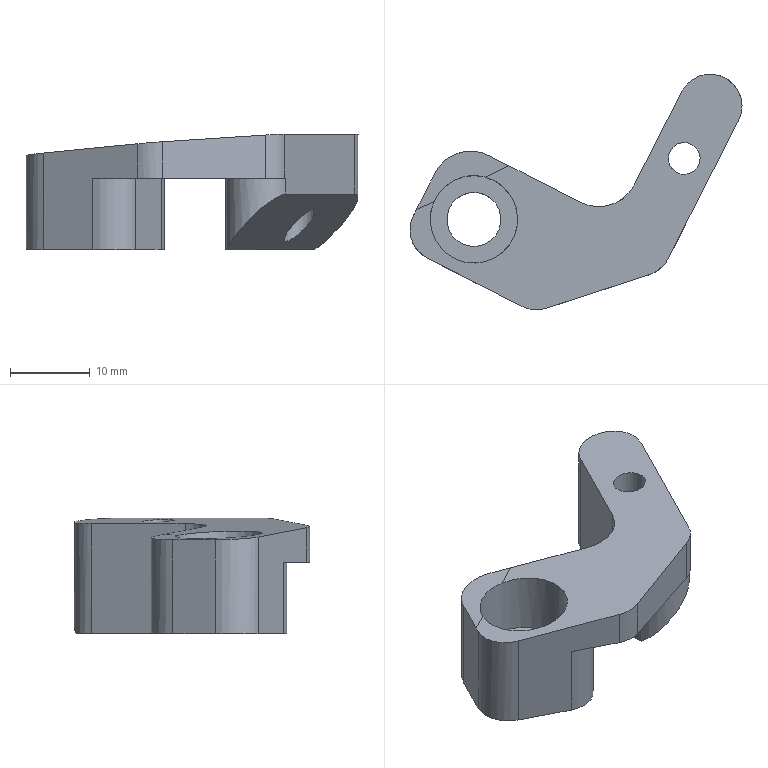Part | STEP file | gslz 2016.10.28-13_id1778_x_t | 1 solid | 26 faces | box 41.743 x 29.62 x 14.53 mm | volume 4507 mm3 | plane 14 | cylinder 12 | commonest cylinder face diameters 8 x7 10 x2 4 x1 6.8 x1 11 x1